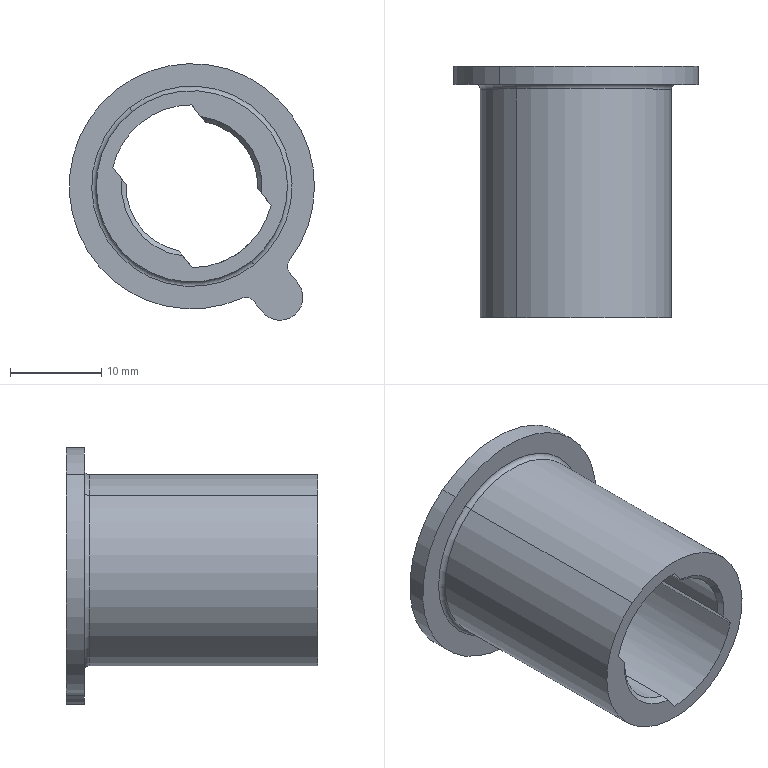Part | SolidWorks | features BaseBody 1 | 1 solid | 36 faces | box 26.8 x 27.5 x 28.043 mm | volume 3609 mm3 | cylinder 15 | plane 9 | cone 8 | torus 2 | sphere 2 | commonest cylinder face diameters 17.8 x3 2 x2 5 x2 14.4 x2 18 x2 20.9 x2
STEP:
#1=CARTESIAN_POINT('',(223.907,99.5,7.051));
#2=VERTEX_POINT('',#1);
#3=CARTESIAN_POINT('',(235.093,99.5,-7.051));
#4=VERTEX_POINT('',#3);
#5=CARTESIAN_POINT('',(229.5,99.5,0.));
#6=DIRECTION('',(0.,1.,0.));
#7=DIRECTION('',(0.6215,0.,-0.7834));
#8=AXIS2_PLACEMENT_3D('',#5,#6,#7);
#9=CIRCLE('',#8,9.);
#10=EDGE_CURVE('',#2,#4,#9,.T.);
#11=ORIENTED_EDGE('',*,*,#10,.F.);
#12=CARTESIAN_POINT('',(223.596,100.,7.443));
#13=VERTEX_POINT('',#12);
#14=CARTESIAN_POINT('',(223.596,100.,7.443));
#15=DIRECTION('',(-0.4395,0.7071,0.554));
#16=VECTOR('',#15,1000.);
#17=LINE('',#14,#16);
#18=EDGE_CURVE('',#2,#13,#17,.T.);
#19=ORIENTED_EDGE('',*,*,#18,.T.);
#20=CARTESIAN_POINT('',(235.404,100.,-7.443));
#21=VERTEX_POINT('',#20);
#22=CARTESIAN_POINT('',(229.5,100.,0.));
#23=DIRECTION('',(0.,-1.,0.));
#24=DIRECTION('',(0.6215,0.,-0.7834));
#25=AXIS2_PLACEMENT_3D('',#22,#23,#24);
#26=CIRCLE('',#25,9.5);
#27=EDGE_CURVE('',#21,#13,#26,.T.);
#28=ORIENTED_EDGE('',*,*,#27,.F.);
#29=CARTESIAN_POINT('',(235.404,100.,-7.443));
#30=DIRECTION('',(0.4395,0.7071,-0.554));
#31=VECTOR('',#30,1000.);
#32=LINE('',#29,#31);
#33=EDGE_CURVE('',#4,#21,#32,.T.);
#34=ORIENTED_EDGE('',*,*,#33,.F.);
#35=EDGE_LOOP('',(#11,#19,#28,#34));
#36=FACE_OUTER_BOUND('',#35,.T.);
#37=CARTESIAN_POINT('',(229.5,100.,0.));
#38=DIRECTION('',(0.,1.,0.));
#39=DIRECTION('',(0.6215,0.,-0.7834));
#40=AXIS2_PLACEMENT_3D('',#37,#38,#39);
#41=CONICAL_SURFACE('',#40,9.5,0.7854);
#42=ADVANCED_FACE('',(#36),#41,.F.);
#43=CARTESIAN_POINT('',(235.995,97.5,-8.187));
#44=VERTEX_POINT('',#43);
#45=CARTESIAN_POINT('',(223.005,97.5,8.187));
#46=VERTEX_POINT('',#45);
#47=CARTESIAN_POINT('',(229.5,97.5,0.));
#48=DIRECTION('',(0.,-1.,0.));
#49=DIRECTION('',(-0.6215,0.,0.7834));
#50=AXIS2_PLACEMENT_3D('',#47,#48,#49);
#51=CIRCLE('',#50,10.45);
#52=EDGE_CURVE('',#44,#46,#51,.T.);
#53=ORIENTED_EDGE('',*,*,#52,.F.);
#54=CARTESIAN_POINT('',(236.305,98.,-8.578));
#55=VERTEX_POINT('',#54);
#56=CARTESIAN_POINT('',(236.305,97.5,-8.578));
#57=DIRECTION('',(-0.7834,0.,-0.6215));
#58=DIRECTION('',(-0.6215,0.,0.7834));
#59=AXIS2_PLACEMENT_3D('',#56,#57,#58);
#60=CIRCLE('',#59,0.5);
#61=EDGE_CURVE('',#44,#55,#60,.T.);
#62=ORIENTED_EDGE('',*,*,#61,.T.);
#63=CARTESIAN_POINT('',(222.695,98.,8.578));
#64=VERTEX_POINT('',#63);
#65=CARTESIAN_POINT('',(229.5,98.,0.));
#66=DIRECTION('',(0.,1.,0.));
#67=DIRECTION('',(-0.6215,0.,0.7834));
#68=AXIS2_PLACEMENT_3D('',#65,#66,#67);
#69=CIRCLE('',#68,10.95);
#70=EDGE_CURVE('',#64,#55,#69,.T.);
#71=ORIENTED_EDGE('',*,*,#70,.F.);
#72=CARTESIAN_POINT('',(222.695,97.5,8.578));
#73=DIRECTION('',(0.7834,0.,0.6215));
#74=DIRECTION('',(0.6215,0.,-0.7834));
#75=AXIS2_PLACEMENT_3D('',#72,#73,#74);
#76=CIRCLE('',#75,0.5);
#77=EDGE_CURVE('',#46,#64,#76,.T.);
#78=ORIENTED_EDGE('',*,*,#77,.F.);
#79=EDGE_LOOP('',(#53,#62,#71,#78));
#80=FACE_OUTER_BOUND('',#79,.T.);
#81=CARTESIAN_POINT('',(229.5,97.5,0.));
#82=DIRECTION('',(0.,-1.,0.));
#83=DIRECTION('',(-0.6215,0.,0.7834));
#84=AXIS2_PLACEMENT_3D('',#81,#82,#83);
#85=TOROIDAL_SURFACE('',#84,10.95,0.5);
#86=ADVANCED_FACE('',(#80),#85,.F.);
#87=CARTESIAN_POINT('',(239.133,99.5,-12.143));
#88=VERTEX_POINT('',#87);
#89=CARTESIAN_POINT('',(240.065,100.,-13.318));
#90=VERTEX_POINT('',#89);
#91=CARTESIAN_POINT('',(239.133,102.,-12.143));
#92=DIRECTION('',(0.7834,0.,0.6215));
#93=DIRECTION('',(0.6215,0.,-0.7834));
#94=AXIS2_PLACEMENT_3D('',#91,#92,#93);
#95=CIRCLE('',#94,2.5);
#96=EDGE_CURVE('',#88,#90,#95,.T.);
#97=ORIENTED_EDGE('',*,*,#96,.F.);
#98=CARTESIAN_POINT('',(238.201,100.,-10.968));
#99=VERTEX_POINT('',#98);
#100=CARTESIAN_POINT('',(239.133,102.,-12.143));
#101=DIRECTION('',(-0.7834,0.,-0.6215));
#102=DIRECTION('',(-0.6215,0.,0.7834));
#103=AXIS2_PLACEMENT_3D('',#100,#101,#102);
#104=CIRCLE('',#103,2.5);
#105=EDGE_CURVE('',#88,#99,#104,.T.);
#106=ORIENTED_EDGE('',*,*,#105,.T.);
#107=CARTESIAN_POINT('',(239.133,100.,-12.143));
#108=DIRECTION('',(0.,1.,0.));
#109=DIRECTION('',(0.6215,0.,-0.7834));
#110=AXIS2_PLACEMENT_3D('',#107,#108,#109);
#111=CIRCLE('',#110,1.5);
#112=EDGE_CURVE('',#99,#90,#111,.T.);
#113=ORIENTED_EDGE('',*,*,#112,.T.);
#114=EDGE_LOOP('',(#97,#106,#113));
#115=FACE_OUTER_BOUND('',#114,.T.);
#116=CARTESIAN_POINT('',(239.133,102.,-12.143));
#117=DIRECTION('',(-0.7834,0.,-0.6215));
#118=DIRECTION('',(0.6215,0.,-0.7834));
#119=AXIS2_PLACEMENT_3D('',#116,#117,#118);
#120=SPHERICAL_SURFACE('',#119,2.5);
#121=ADVANCED_FACE('',(#115),#120,.F.);
#122=CARTESIAN_POINT('',(220.843,86.8,2.064));
#123=VERTEX_POINT('',#122);
#124=CARTESIAN_POINT('',(223.969,86.8,6.972));
#125=VERTEX_POINT('',#124);
#126=CARTESIAN_POINT('',(229.5,86.8,0.));
#127=DIRECTION('',(0.,1.,0.));
#128=DIRECTION('',(0.6215,0.,-0.7834));
#129=AXIS2_PLACEMENT_3D('',#126,#127,#128);
#130=CIRCLE('',#129,8.9);
#131=EDGE_CURVE('',#123,#125,#130,.T.);
#132=ORIENTED_EDGE('',*,*,#131,.T.);
#133=CARTESIAN_POINT('',(223.969,72.5,6.972));
#134=VERTEX_POINT('',#133);
#135=CARTESIAN_POINT('',(223.969,100.,6.972));
#136=DIRECTION('',(0.,-1.,0.));
#137=VECTOR('',#136,1000.);
#138=LINE('',#135,#137);
#139=EDGE_CURVE('',#125,#134,#138,.T.);
#140=ORIENTED_EDGE('',*,*,#139,.T.);
#141=CARTESIAN_POINT('',(220.843,72.5,2.064));
#142=VERTEX_POINT('',#141);
#143=CARTESIAN_POINT('',(229.5,72.5,0.));
#144=DIRECTION('',(0.,-1.,0.));
#145=DIRECTION('',(-0.6215,0.,0.7834));
#146=AXIS2_PLACEMENT_3D('',#143,#144,#145);
#147=CIRCLE('',#146,8.9);
#148=EDGE_CURVE('',#134,#142,#147,.T.);
#149=ORIENTED_EDGE('',*,*,#148,.T.);
#150=CARTESIAN_POINT('',(220.843,100.,2.064));
#151=DIRECTION('',(0.,-1.,0.));
#152=VECTOR('',#151,1000.);
#153=LINE('',#150,#152);
#154=EDGE_CURVE('',#123,#142,#153,.T.);
#155=ORIENTED_EDGE('',*,*,#154,.F.);
#156=EDGE_LOOP('',(#132,#140,#149,#155));
#157=FACE_OUTER_BOUND('',#156,.T.);
#158=CARTESIAN_POINT('',(229.5,100.,0.));
#159=DIRECTION('',(0.,-1.,0.));
#160=DIRECTION('',(-0.6215,0.,0.7834));
#161=AXIS2_PLACEMENT_3D('',#158,#159,#160);
#162=CYLINDRICAL_SURFACE('',#161,8.9);
#163=ADVANCED_FACE('',(#157),#162,.F.);
#164=CARTESIAN_POINT('',(241.092,98.,-10.589));
#165=VERTEX_POINT('',#164);
#166=CARTESIAN_POINT('',(240.687,98.,-14.102));
#167=VERTEX_POINT('',#166);
#168=CARTESIAN_POINT('',(239.133,98.,-12.143));
#169=DIRECTION('',(0.,1.,0.));
#170=DIRECTION('',(-0.6215,0.,0.7834));
#171=AXIS2_PLACEMENT_3D('',#168,#169,#170);
#172=CIRCLE('',#171,2.5);
#173=EDGE_CURVE('',#165,#167,#172,.T.);
#174=ORIENTED_EDGE('',*,*,#173,.T.);
#175=CARTESIAN_POINT('',(240.687,100.,-14.102));
#176=VERTEX_POINT('',#175);
#177=CARTESIAN_POINT('',(240.687,56.718,-14.102));
#178=DIRECTION('',(0.,1.,0.));
#179=VECTOR('',#178,1000.);
#180=LINE('',#177,#179);
#181=EDGE_CURVE('',#167,#176,#180,.T.);
#182=ORIENTED_EDGE('',*,*,#181,.T.);
#183=CARTESIAN_POINT('',(241.092,100.,-10.589));
#184=VERTEX_POINT('',#183);
#185=CARTESIAN_POINT('',(239.133,100.,-12.143));
#186=DIRECTION('',(0.,1.,0.));
#187=DIRECTION('',(-0.6215,0.,0.7834));
#188=AXIS2_PLACEMENT_3D('',#185,#186,#187);
#189=CIRCLE('',#188,2.5);
#190=EDGE_CURVE('',#184,#176,#189,.T.);
#191=ORIENTED_EDGE('',*,*,#190,.F.);
#192=CARTESIAN_POINT('',(241.092,56.718,-10.589));
#193=DIRECTION('',(0.,1.,0.));
#194=VECTOR('',#193,1000.);
#195=LINE('',#192,#194);
#196=EDGE_CURVE('',#165,#184,#195,.T.);
#197=ORIENTED_EDGE('',*,*,#196,.F.);
#198=EDGE_LOOP('',(#174,#182,#191,#197));
#199=FACE_OUTER_BOUND('',#198,.T.);
#200=CARTESIAN_POINT('',(239.133,56.718,-12.143));
#201=DIRECTION('',(0.,1.,0.));
#202=DIRECTION('',(0.6215,0.,-0.7834));
#203=AXIS2_PLACEMENT_3D('',#200,#201,#202);
#204=CYLINDRICAL_SURFACE('',#203,2.5);
#205=ADVANCED_FACE('',(#199),#204,.T.);
#206=CARTESIAN_POINT('',(229.46,86.8,8.9));
#207=VERTEX_POINT('',#206);
#208=CARTESIAN_POINT('',(229.5,86.8,0.));
#209=DIRECTION('',(0.,1.,0.));
#210=DIRECTION('',(0.6215,0.,-0.7834));
#211=AXIS2_PLACEMENT_3D('',#208,#209,#210);
#212=CIRCLE('',#211,8.9);
#213=EDGE_CURVE('',#125,#207,#212,.T.);
#214=ORIENTED_EDGE('',*,*,#213,.F.);
#215=CARTESIAN_POINT('',(223.907,86.9,7.051));
#216=VERTEX_POINT('',#215);
#217=CARTESIAN_POINT('',(223.907,86.9,7.051));
#218=DIRECTION('',(-0.4395,0.7071,0.554));
#219=VECTOR('',#218,1000.);
#220=LINE('',#217,#219);
#221=EDGE_CURVE('',#125,#216,#220,.T.);
#222=ORIENTED_EDGE('',*,*,#221,.T.);
#223=CARTESIAN_POINT('',(235.093,86.9,-7.051));
#224=VERTEX_POINT('',#223);
#225=CARTESIAN_POINT('',(229.5,86.9,0.));
#226=DIRECTION('',(0.,-1.,0.));
#227=DIRECTION('',(-0.6215,0.,0.7834));
#228=AXIS2_PLACEMENT_3D('',#225,#226,#227);
#229=CIRCLE('',#228,9.);
#230=EDGE_CURVE('',#224,#216,#229,.T.);
#231=ORIENTED_EDGE('',*,*,#230,.F.);
#232=CARTESIAN_POINT('',(235.031,86.8,-6.972));
#233=VERTEX_POINT('',#232);
#234=CARTESIAN_POINT('',(235.093,86.9,-7.051));
#235=DIRECTION('',(0.4395,0.7071,-0.554));
#236=VECTOR('',#235,1000.);
#237=LINE('',#234,#236);
#238=EDGE_CURVE('',#233,#224,#237,.T.);
#239=ORIENTED_EDGE('',*,*,#238,.F.);
#240=CARTESIAN_POINT('',(238.157,86.8,-2.064));
#241=VERTEX_POINT('',#240);
#242=CARTESIAN_POINT('',(229.5,86.8,0.));
#243=DIRECTION('',(0.,1.,0.));
#244=DIRECTION('',(0.6215,0.,-0.7834));
#245=AXIS2_PLACEMENT_3D('',#242,#243,#244);
#246=CIRCLE('',#245,8.9);
#247=EDGE_CURVE('',#241,#233,#246,.T.);
#248=ORIENTED_EDGE('',*,*,#247,.F.);
#249=CARTESIAN_POINT('',(237.998,86.6,-1.863));
#250=VERTEX_POINT('',#249);
#251=CARTESIAN_POINT('',(237.998,86.6,-1.863));
#252=CARTESIAN_POINT('',(238.051,86.666,-1.93));
#253=CARTESIAN_POINT('',(238.105,86.733,-1.997));
#254=CARTESIAN_POINT('',(238.157,86.8,-2.064));
#255=B_SPLINE_CURVE_WITH_KNOTS('',3,(#251,#252,#253,#254),.UNSPECIFIED.,.F.,.F.,(4,4),(0.004277,0.004601),.UNSPECIFIED.);
#256=EDGE_CURVE('',#250,#241,#255,.T.);
#257=ORIENTED_EDGE('',*,*,#256,.F.);
#258=CARTESIAN_POINT('',(229.619,86.6,8.699));
#259=VERTEX_POINT('',#258);
#260=CARTESIAN_POINT('',(229.5,86.6,0.));
#261=DIRECTION('',(0.,-1.,0.));
#262=DIRECTION('',(-0.6215,0.,0.7834));
#263=AXIS2_PLACEMENT_3D('',#260,#261,#262);
#264=CIRCLE('',#263,8.7);
#265=EDGE_CURVE('',#250,#259,#264,.T.);
#266=ORIENTED_EDGE('',*,*,#265,.T.);
#267=CARTESIAN_POINT('',(229.46,86.8,8.9));
#268=CARTESIAN_POINT('',(229.513,86.733,8.833));
#269=CARTESIAN_POINT('',(229.566,86.666,8.766));
#270=CARTESIAN_POINT('',(229.619,86.6,8.699));
#271=B_SPLINE_CURVE_WITH_KNOTS('',3,(#267,#268,#269,#270),.UNSPECIFIED.,.F.,.F.,(4,4),(0.004066,0.00439),.UNSPECIFIED.);
#272=EDGE_CURVE('',#207,#259,#271,.T.);
#273=ORIENTED_EDGE('',*,*,#272,.F.);
#274=EDGE_LOOP('',(#214,#222,#231,#239,#248,#257,#266,#273));
#275=FACE_OUTER_BOUND('',#274,.T.);
#276=CARTESIAN_POINT('',(229.5,86.9,0.));
#277=DIRECTION('',(0.,1.,0.));
#278=DIRECTION('',(0.6215,0.,-0.7834));
#279=AXIS2_PLACEMENT_3D('',#276,#277,#278);
#280=CONICAL_SURFACE('',#279,9.,0.7854);
#281=ADVANCED_FACE('',(#275),#280,.F.);
#282=ORIENTED_EDGE('',*,*,#10,.T.);
#283=CARTESIAN_POINT('',(235.093,72.5,-7.051));
#284=DIRECTION('',(0.,-1.,0.));
#285=VECTOR('',#284,1000.);
#286=LINE('',#283,#285);
#287=EDGE_CURVE('',#4,#224,#286,.T.);
#288=ORIENTED_EDGE('',*,*,#287,.T.);
#289=ORIENTED_EDGE('',*,*,#230,.T.);
#290=CARTESIAN_POINT('',(223.907,72.5,7.051));
#291=DIRECTION('',(0.,-1.,0.));
#292=VECTOR('',#291,1000.);
#293=LINE('',#290,#292);
#294=EDGE_CURVE('',#2,#216,#293,.T.);
#295=ORIENTED_EDGE('',*,*,#294,.F.);
#296=EDGE_LOOP('',(#282,#288,#289,#295));
#297=FACE_OUTER_BOUND('',#296,.T.);
#298=CARTESIAN_POINT('',(229.5,72.5,0.));
#299=DIRECTION('',(0.,-1.,0.));
#300=DIRECTION('',(-0.6215,0.,0.7834));
#301=AXIS2_PLACEMENT_3D('',#298,#299,#300);
#302=CYLINDRICAL_SURFACE('',#301,9.);
#303=ADVANCED_FACE('',(#297),#302,.F.);
#304=CARTESIAN_POINT('',(240.13,100.,-8.159));
#305=VERTEX_POINT('',#304);
#306=CARTESIAN_POINT('',(221.172,100.,10.498));
#307=VERTEX_POINT('',#306);
#308=CARTESIAN_POINT('',(229.5,100.,0.));
#309=DIRECTION('',(0.,-1.,0.));
#310=DIRECTION('',(-0.6215,0.,0.7834));
#311=AXIS2_PLACEMENT_3D('',#308,#309,#310);
#312=CIRCLE('',#311,13.4);
#313=EDGE_CURVE('',#305,#307,#312,.T.);
#314=ORIENTED_EDGE('',*,*,#313,.T.);
#315=CARTESIAN_POINT('',(221.172,98.,10.498));
#316=VERTEX_POINT('',#315);
#317=CARTESIAN_POINT('',(221.172,72.5,10.498));
#318=DIRECTION('',(0.,-1.,0.));
#319=VECTOR('',#318,1000.);
#320=LINE('',#317,#319);
#321=EDGE_CURVE('',#307,#316,#320,.T.);
#322=ORIENTED_EDGE('',*,*,#321,.T.);
#323=CARTESIAN_POINT('',(240.13,98.,-8.159));
#324=VERTEX_POINT('',#323);
#325=CARTESIAN_POINT('',(229.5,98.,0.));
#326=DIRECTION('',(0.,-1.,0.));
#327=DIRECTION('',(-0.6215,0.,0.7834));
#328=AXIS2_PLACEMENT_3D('',#325,#326,#327);
#329=CIRCLE('',#328,13.4);
#330=EDGE_CURVE('',#324,#316,#329,.T.);
#331=ORIENTED_EDGE('',*,*,#330,.F.);
#332=CARTESIAN_POINT('',(240.13,72.5,-8.159));
#333=DIRECTION('',(0.,1.,0.));
#334=VECTOR('',#333,1000.);
#335=LINE('',#332,#334);
#336=EDGE_CURVE('',#324,#305,#335,.T.);
#337=ORIENTED_EDGE('',*,*,#336,.T.);
#338=EDGE_LOOP('',(#314,#322,#331,#337));
#339=FACE_OUTER_BOUND('',#338,.T.);
#340=CARTESIAN_POINT('',(229.5,72.5,0.));
#341=DIRECTION('',(0.,-1.,0.));
#342=DIRECTION('',(-0.6215,0.,0.7834));
#343=AXIS2_PLACEMENT_3D('',#340,#341,#342);
#344=CYLINDRICAL_SURFACE('',#343,13.4);
#345=ADVANCED_FACE('',(#339),#344,.T.);
#346=CARTESIAN_POINT('',(229.5,97.5,0.));
#347=DIRECTION('',(0.,-1.,0.));
#348=DIRECTION('',(-0.6215,0.,0.7834));
#349=AXIS2_PLACEMENT_3D('',#346,#347,#348);
#350=CIRCLE('',#349,10.45);
#351=EDGE_CURVE('',#46,#44,#350,.T.);
#352=ORIENTED_EDGE('',*,*,#351,.T.);
#353=CARTESIAN_POINT('',(235.995,72.5,-8.187));
#354=VERTEX_POINT('',#353);
#355=CARTESIAN_POINT('',(235.995,72.5,-8.187));
#356=DIRECTION('',(0.,-1.,0.));
#357=VECTOR('',#356,1000.);
#358=LINE('',#355,#357);
#359=EDGE_CURVE('',#44,#354,#358,.T.);
#360=ORIENTED_EDGE('',*,*,#359,.T.);
#361=CARTESIAN_POINT('',(223.005,72.5,8.187));
#362=VERTEX_POINT('',#361);
#363=CARTESIAN_POINT('',(229.5,72.5,0.));
#364=DIRECTION('',(0.,-1.,0.));
#365=DIRECTION('',(-0.6215,0.,0.7834));
#366=AXIS2_PLACEMENT_3D('',#363,#364,#365);
#367=CIRCLE('',#366,10.45);
#368=EDGE_CURVE('',#362,#354,#367,.T.);
#369=ORIENTED_EDGE('',*,*,#368,.F.);
#370=CARTESIAN_POINT('',(223.005,72.5,8.187));
#371=DIRECTION('',(0.,-1.,0.));
#372=VECTOR('',#371,1000.);
#373=LINE('',#370,#372);
#374=EDGE_CURVE('',#46,#362,#373,.T.);
#375=ORIENTED_EDGE('',*,*,#374,.F.);
#376=EDGE_LOOP('',(#352,#360,#369,#375));
#377=FACE_OUTER_BOUND('',#376,.T.);
#378=CARTESIAN_POINT('',(229.5,72.5,0.));
#379=DIRECTION('',(0.,-1.,0.));
#380=DIRECTION('',(-0.6215,0.,0.7834));
#381=AXIS2_PLACEMENT_3D('',#378,#379,#380);
#382=CYLINDRICAL_SURFACE('',#381,10.45);
#383=ADVANCED_FACE('',(#377),#382,.T.);
#384=CARTESIAN_POINT('',(222.303,85.734,0.222));
#385=VERTEX_POINT('',#384);
#386=CARTESIAN_POINT('',(222.303,73.,0.222));
#387=VERTEX_POINT('',#386);
#388=CARTESIAN_POINT('',(222.303,100.,0.222));
#389=DIRECTION('',(0.,-1.,0.));
#390=VECTOR('',#389,1000.);
#391=LINE('',#388,#390);
#392=EDGE_CURVE('',#385,#387,#391,.T.);
#393=ORIENTED_EDGE('',*,*,#392,.T.);
#394=CARTESIAN_POINT('',(228.079,73.,-7.058));
#395=VERTEX_POINT('',#394);
#396=CARTESIAN_POINT('',(229.5,73.,0.));
#397=DIRECTION('',(0.,-1.,0.));
#398=DIRECTION('',(-0.6215,0.,0.7834));
#399=AXIS2_PLACEMENT_3D('',#396,#397,#398);
#400=CIRCLE('',#399,7.2);
#401=EDGE_CURVE('',#387,#395,#400,.T.);
#402=ORIENTED_EDGE('',*,*,#401,.T.);
#403=CARTESIAN_POINT('',(228.079,85.734,-7.058));
#404=VERTEX_POINT('',#403);
#405=CARTESIAN_POINT('',(228.079,100.,-7.058));
#406=DIRECTION('',(0.,-1.,0.));
#407=VECTOR('',#406,1000.);
#408=LINE('',#405,#407);
#409=EDGE_CURVE('',#404,#395,#408,.T.);
#410=ORIENTED_EDGE('',*,*,#409,.F.);
#411=CARTESIAN_POINT('',(229.5,85.734,0.));
#412=DIRECTION('',(0.,-1.,0.));
#413=DIRECTION('',(-0.6215,0.,0.7834));
#414=AXIS2_PLACEMENT_3D('',#411,#412,#413);
#415=CIRCLE('',#414,7.2);
#416=EDGE_CURVE('',#385,#404,#415,.T.);
#417=ORIENTED_EDGE('',*,*,#416,.F.);
#418=EDGE_LOOP('',(#393,#402,#410,#417));
#419=FACE_OUTER_BOUND('',#418,.T.);
#420=CARTESIAN_POINT('',(229.5,72.5,0.));
#421=DIRECTION('',(0.,-1.,0.));
#422=DIRECTION('',(-0.6215,0.,0.7834));
#423=AXIS2_PLACEMENT_3D('',#420,#421,#422);
#424=CYLINDRICAL_SURFACE('',#423,7.2);
#425=ADVANCED_FACE('',(#419),#424,.F.);
#426=CARTESIAN_POINT('',(229.381,86.6,-8.699));
#427=VERTEX_POINT('',#426);
#428=CARTESIAN_POINT('',(229.381,86.6,-8.699));
#429=CARTESIAN_POINT('',(228.952,86.292,-8.159));
#430=CARTESIAN_POINT('',(228.519,85.997,-7.612));
#431=CARTESIAN_POINT('',(228.079,85.734,-7.058));
#432=B_SPLINE_CURVE_WITH_KNOTS('',3,(#428,#429,#430,#431),.UNSPECIFIED.,.F.,.F.,(4,4),(0.003137,0.005403),.UNSPECIFIED.);
#433=EDGE_CURVE('',#427,#404,#432,.T.);
#434=ORIENTED_EDGE('',*,*,#433,.F.);
#435=CARTESIAN_POINT('',(221.002,86.6,1.863));
#436=VERTEX_POINT('',#435);
#437=CARTESIAN_POINT('',(229.5,86.6,0.));
#438=DIRECTION('',(0.,-1.,0.));
#439=DIRECTION('',(-0.6215,0.,0.7834));
#440=AXIS2_PLACEMENT_3D('',#437,#438,#439);
#441=CIRCLE('',#440,8.7);
#442=EDGE_CURVE('',#436,#427,#441,.T.);
#443=ORIENTED_EDGE('',*,*,#442,.F.);
#444=CARTESIAN_POINT('',(222.303,85.734,0.222));
#445=CARTESIAN_POINT('',(221.864,85.997,0.7756));
#446=CARTESIAN_POINT('',(221.431,86.291,1.322));
#447=CARTESIAN_POINT('',(221.002,86.6,1.863));
#448=B_SPLINE_CURVE_WITH_KNOTS('',3,(#444,#445,#446,#447),.UNSPECIFIED.,.F.,.F.,(4,4),(0.002935,0.005196),.UNSPECIFIED.);
#449=EDGE_CURVE('',#385,#436,#448,.T.);
#450=ORIENTED_EDGE('',*,*,#449,.F.);
#451=ORIENTED_EDGE('',*,*,#416,.T.);
#452=EDGE_LOOP('',(#434,#443,#450,#451));
#453=FACE_OUTER_BOUND('',#452,.T.);
#454=CARTESIAN_POINT('',(229.5,86.6,0.));
#455=DIRECTION('',(0.,1.,0.));
#456=DIRECTION('',(0.6215,0.,-0.7834));
#457=AXIS2_PLACEMENT_3D('',#454,#455,#456);
#458=CONICAL_SURFACE('',#457,8.7,1.047);
#459=ADVANCED_FACE('',(#453),#458,.F.);
#460=CARTESIAN_POINT('',(236.697,85.734,-0.222));
#461=VERTEX_POINT('',#460);
#462=CARTESIAN_POINT('',(236.697,73.,-0.222));
#463=VERTEX_POINT('',#462);
#464=CARTESIAN_POINT('',(236.697,100.,-0.222));
#465=DIRECTION('',(0.,-1.,0.));
#466=VECTOR('',#465,1000.);
#467=LINE('',#464,#466);
#468=EDGE_CURVE('',#461,#463,#467,.T.);
#469=ORIENTED_EDGE('',*,*,#468,.T.);
#470=CARTESIAN_POINT('',(230.921,73.,7.058));
#471=VERTEX_POINT('',#470);
#472=CARTESIAN_POINT('',(229.5,73.,0.));
#473=DIRECTION('',(0.,-1.,0.));
#474=DIRECTION('',(-0.6215,0.,0.7834));
#475=AXIS2_PLACEMENT_3D('',#472,#473,#474);
#476=CIRCLE('',#475,7.2);
#477=EDGE_CURVE('',#463,#471,#476,.T.);
#478=ORIENTED_EDGE('',*,*,#477,.T.);
#479=CARTESIAN_POINT('',(230.921,85.734,7.058));
#480=VERTEX_POINT('',#479);
#481=CARTESIAN_POINT('',(230.921,100.,7.058));
#482=DIRECTION('',(0.,-1.,0.));
#483=VECTOR('',#482,1000.);
#484=LINE('',#481,#483);
#485=EDGE_CURVE('',#480,#471,#484,.T.);
#486=ORIENTED_EDGE('',*,*,#485,.F.);
#487=CARTESIAN_POINT('',(229.5,85.734,0.));
#488=DIRECTION('',(0.,-1.,0.));
#489=DIRECTION('',(-0.6215,0.,0.7834));
#490=AXIS2_PLACEMENT_3D('',#487,#488,#489);
#491=CIRCLE('',#490,7.2);
#492=EDGE_CURVE('',#461,#480,#491,.T.);
#493=ORIENTED_EDGE('',*,*,#492,.F.);
#494=EDGE_LOOP('',(#469,#478,#486,#493));
#495=FACE_OUTER_BOUND('',#494,.T.);
#496=CARTESIAN_POINT('',(229.5,72.5,0.));
#497=DIRECTION('',(0.,-1.,0.));
#498=DIRECTION('',(-0.6215,0.,0.7834));
#499=AXIS2_PLACEMENT_3D('',#496,#497,#498);
#500=CYLINDRICAL_SURFACE('',#499,7.2);
#501=ADVANCED_FACE('',(#495),#500,.F.);
#502=CARTESIAN_POINT('',(230.46,72.5,7.64));
#503=VERTEX_POINT('',#502);
#504=CARTESIAN_POINT('',(229.46,72.5,8.9));
#505=VERTEX_POINT('',#504);
#506=CARTESIAN_POINT('',(230.921,72.5,7.058));
#507=DIRECTION('',(-0.6215,0.,0.7834));
#508=VECTOR('',#507,1000.);
#509=LINE('',#506,#508);
#510=EDGE_CURVE('',#503,#505,#509,.T.);
#511=ORIENTED_EDGE('',*,*,#510,.F.);
#512=CARTESIAN_POINT('',(237.158,72.5,-0.8036));
#513=VERTEX_POINT('',#512);
#514=CARTESIAN_POINT('',(229.5,72.5,0.));
#515=DIRECTION('',(0.,1.,0.));
#516=DIRECTION('',(-0.6215,0.,0.7834));
#517=AXIS2_PLACEMENT_3D('',#514,#515,#516);
#518=CIRCLE('',#517,7.7);
#519=EDGE_CURVE('',#503,#513,#518,.T.);
#520=ORIENTED_EDGE('',*,*,#519,.T.);
#521=CARTESIAN_POINT('',(238.157,72.5,-2.064));
#522=VERTEX_POINT('',#521);
#523=CARTESIAN_POINT('',(236.697,72.5,-0.222));
#524=DIRECTION('',(-0.6215,0.,0.7834));
#525=VECTOR('',#524,1000.);
#526=LINE('',#523,#525);
#527=EDGE_CURVE('',#522,#513,#526,.T.);
#528=ORIENTED_EDGE('',*,*,#527,.F.);
#529=CARTESIAN_POINT('',(229.54,72.5,-8.9));
#530=VERTEX_POINT('',#529);
#531=CARTESIAN_POINT('',(229.5,72.5,0.));
#532=DIRECTION('',(0.,-1.,0.));
#533=DIRECTION('',(-0.6215,0.,0.7834));
#534=AXIS2_PLACEMENT_3D('',#531,#532,#533);
#535=CIRCLE('',#534,8.9);
#536=EDGE_CURVE('',#530,#522,#535,.T.);
#537=ORIENTED_EDGE('',*,*,#536,.F.);
#538=CARTESIAN_POINT('',(228.54,72.5,-7.64));
#539=VERTEX_POINT('',#538);
#540=CARTESIAN_POINT('',(228.079,72.5,-7.058));
#541=DIRECTION('',(0.6215,0.,-0.7834));
#542=VECTOR('',#541,1000.);
#543=LINE('',#540,#542);
#544=EDGE_CURVE('',#539,#530,#543,.T.);
#545=ORIENTED_EDGE('',*,*,#544,.F.);
#546=CARTESIAN_POINT('',(221.842,72.5,0.8036));
#547=VERTEX_POINT('',#546);
#548=CARTESIAN_POINT('',(229.5,72.5,0.));
#549=DIRECTION('',(0.,1.,0.));
#550=DIRECTION('',(-0.6215,0.,0.7834));
#551=AXIS2_PLACEMENT_3D('',#548,#549,#550);
#552=CIRCLE('',#551,7.7);
#553=EDGE_CURVE('',#539,#547,#552,.T.);
#554=ORIENTED_EDGE('',*,*,#553,.T.);
#555=CARTESIAN_POINT('',(222.303,72.5,0.222));
#556=DIRECTION('',(0.6215,0.,-0.7834));
#557=VECTOR('',#556,1000.);
#558=LINE('',#555,#557);
#559=EDGE_CURVE('',#142,#547,#558,.T.);
#560=ORIENTED_EDGE('',*,*,#559,.F.);
#561=ORIENTED_EDGE('',*,*,#148,.F.);
#562=CARTESIAN_POINT('',(229.5,72.5,0.));
#563=DIRECTION('',(0.,-1.,0.));
#564=DIRECTION('',(-0.6215,0.,0.7834));
#565=AXIS2_PLACEMENT_3D('',#562,#563,#564);
#566=CIRCLE('',#565,8.9);
#567=EDGE_CURVE('',#505,#134,#566,.T.);
#568=ORIENTED_EDGE('',*,*,#567,.F.);
#569=EDGE_LOOP('',(#511,#520,#528,#537,#545,#554,#560,#561,#568));
#570=FACE_BOUND('',#569,.T.);
#571=ORIENTED_EDGE('',*,*,#368,.T.);
#572=CARTESIAN_POINT('',(229.5,72.5,0.));
#573=DIRECTION('',(0.,-1.,0.));
#574=DIRECTION('',(-0.6215,0.,0.7834));
#575=AXIS2_PLACEMENT_3D('',#572,#573,#574);
#576=CIRCLE('',#575,10.45);
#577=EDGE_CURVE('',#354,#362,#576,.T.);
#578=ORIENTED_EDGE('',*,*,#577,.T.);
#579=EDGE_LOOP('',(#571,#578));
#580=FACE_OUTER_BOUND('',#579,.T.);
#581=CARTESIAN_POINT('',(223.859,72.5,-4.475));
#582=DIRECTION('',(0.,-1.,0.));
#583=DIRECTION('',(-0.6215,0.,0.7834));
#584=AXIS2_PLACEMENT_3D('',#581,#582,#583);
#585=PLANE('',#584);
#586=ADVANCED_FACE('',(#570,#580),#585,.T.);
#587=ORIENTED_EDGE('',*,*,#359,.F.);
#588=ORIENTED_EDGE('',*,*,#52,.T.);
#589=ORIENTED_EDGE('',*,*,#374,.T.);
#590=ORIENTED_EDGE('',*,*,#577,.F.);
#591=EDGE_LOOP('',(#587,#588,#589,#590));
#592=FACE_OUTER_BOUND('',#591,.T.);
#593=CARTESIAN_POINT('',(229.5,72.5,0.));
#594=DIRECTION('',(0.,-1.,0.));
#595=DIRECTION('',(-0.6215,0.,0.7834));
#596=AXIS2_PLACEMENT_3D('',#593,#594,#595);
#597=CYLINDRICAL_SURFACE('',#596,10.45);
#598=ADVANCED_FACE('',(#592),#597,.T.);
#599=ORIENTED_EDGE('',*,*,#70,.T.);
#600=CARTESIAN_POINT('',(229.5,98.,0.));
#601=DIRECTION('',(0.,1.,0.));
#602=DIRECTION('',(-0.6215,0.,0.7834));
#603=AXIS2_PLACEMENT_3D('',#600,#601,#602);
#604=CIRCLE('',#603,10.95);
#605=EDGE_CURVE('',#55,#64,#604,.T.);
#606=ORIENTED_EDGE('',*,*,#605,.T.);
#607=EDGE_LOOP('',(#599,#606));
#608=FACE_BOUND('',#607,.T.);
#609=CARTESIAN_POINT('',(240.14,98.,-9.389));
#610=VERTEX_POINT('',#609);
#611=CARTESIAN_POINT('',(239.64,98.,-8.76));
#612=DIRECTION('',(0.6215,0.,-0.7834));
#613=VECTOR('',#612,1000.);
#614=LINE('',#611,#613);
#615=EDGE_CURVE('',#610,#165,#614,.T.);
#616=ORIENTED_EDGE('',*,*,#615,.F.);
#617=CARTESIAN_POINT('',(240.923,98.,-8.768));
#618=DIRECTION('',(0.,1.,0.));
#619=DIRECTION('',(-0.6215,0.,0.7834));
#620=AXIS2_PLACEMENT_3D('',#617,#618,#619);
#621=CIRCLE('',#620,1.);
#622=EDGE_CURVE('',#610,#324,#621,.T.);
#623=ORIENTED_EDGE('',*,*,#622,.T.);
#624=ORIENTED_EDGE('',*,*,#330,.T.);
#625=CARTESIAN_POINT('',(235.027,98.,-12.207));
#626=VERTEX_POINT('',#625);
#627=CARTESIAN_POINT('',(229.5,98.,0.));
#628=DIRECTION('',(0.,-1.,0.));
#629=DIRECTION('',(-0.6215,0.,0.7834));
#630=AXIS2_PLACEMENT_3D('',#627,#628,#629);
#631=CIRCLE('',#630,13.4);
#632=EDGE_CURVE('',#316,#626,#631,.T.);
#633=ORIENTED_EDGE('',*,*,#632,.T.);
#634=CARTESIAN_POINT('',(236.223,98.,-12.497));
#635=VERTEX_POINT('',#634);
#636=CARTESIAN_POINT('',(235.439,98.,-13.118));
#637=DIRECTION('',(0.,1.,0.));
#638=DIRECTION('',(-0.6215,0.,0.7834));
#639=AXIS2_PLACEMENT_3D('',#636,#637,#638);
#640=CIRCLE('',#639,1.);
#641=EDGE_CURVE('',#626,#635,#640,.T.);
#642=ORIENTED_EDGE('',*,*,#641,.T.);
#643=CARTESIAN_POINT('',(237.175,98.,-13.697));
#644=VERTEX_POINT('',#643);
#645=CARTESIAN_POINT('',(235.723,98.,-11.867));
#646=DIRECTION('',(-0.6215,0.,0.7834));
#647=VECTOR('',#646,1000.);
#648=LINE('',#645,#647);
#649=EDGE_CURVE('',#644,#635,#648,.T.);
#650=ORIENTED_EDGE('',*,*,#649,.F.);
#651=CARTESIAN_POINT('',(239.133,98.,-12.143));
#652=DIRECTION('',(0.,1.,0.));
#653=DIRECTION('',(-0.6215,0.,0.7834));
#654=AXIS2_PLACEMENT_3D('',#651,#652,#653);
#655=CIRCLE('',#654,2.5);
#656=EDGE_CURVE('',#167,#644,#655,.T.);
#657=ORIENTED_EDGE('',*,*,#656,.F.);
#658=ORIENTED_EDGE('',*,*,#173,.F.);
#659=EDGE_LOOP('',(#616,#623,#624,#633,#642,#650,#657,#658));
#660=FACE_OUTER_BOUND('',#659,.T.);
#661=CARTESIAN_POINT('',(221.313,98.,-6.495));
#662=DIRECTION('',(0.,-1.,0.));
#663=DIRECTION('',(-0.6215,0.,0.7834));
#664=AXIS2_PLACEMENT_3D('',#661,#662,#663);
#665=PLANE('',#664);
#666=ADVANCED_FACE('',(#608,#660),#665,.T.);
#667=ORIENTED_EDGE('',*,*,#321,.F.);
#668=CARTESIAN_POINT('',(235.027,100.,-12.207));
#669=VERTEX_POINT('',#668);
#670=CARTESIAN_POINT('',(229.5,100.,0.));
#671=DIRECTION('',(0.,-1.,0.));
#672=DIRECTION('',(-0.6215,0.,0.7834));
#673=AXIS2_PLACEMENT_3D('',#670,#671,#672);
#674=CIRCLE('',#673,13.4);
#675=EDGE_CURVE('',#307,#669,#674,.T.);
#676=ORIENTED_EDGE('',*,*,#675,.T.);
#677=CARTESIAN_POINT('',(235.027,72.5,-12.207));
#678=DIRECTION('',(0.,-1.,0.));
#679=VECTOR('',#678,1000.);
#680=LINE('',#677,#679);
#681=EDGE_CURVE('',#669,#626,#680,.T.);
#682=ORIENTED_EDGE('',*,*,#681,.T.);
#683=ORIENTED_EDGE('',*,*,#632,.F.);
#684=EDGE_LOOP('',(#667,#676,#682,#683));
#685=FACE_OUTER_BOUND('',#684,.T.);
#686=CARTESIAN_POINT('',(229.5,72.5,0.));
#687=DIRECTION('',(0.,-1.,0.));
#688=DIRECTION('',(-0.6215,0.,0.7834));
#689=AXIS2_PLACEMENT_3D('',#686,#687,#688);
#690=CYLINDRICAL_SURFACE('',#689,13.4);
#691=ADVANCED_FACE('',(#685),#690,.T.);
#692=ORIENTED_EDGE('',*,*,#27,.T.);
#693=CARTESIAN_POINT('',(229.5,100.,0.));
#694=DIRECTION('',(0.,-1.,0.));
#695=DIRECTION('',(0.6215,0.,-0.7834));
#696=AXIS2_PLACEMENT_3D('',#693,#694,#695);
#697=CIRCLE('',#696,9.5);
#698=EDGE_CURVE('',#13,#21,#697,.T.);
#699=ORIENTED_EDGE('',*,*,#698,.T.);
#700=EDGE_LOOP('',(#692,#699));
#701=FACE_BOUND('',#700,.T.);
#702=CARTESIAN_POINT('',(239.133,100.,-12.143));
#703=DIRECTION('',(0.,1.,0.));
#704=DIRECTION('',(0.6215,0.,-0.7834));
#705=AXIS2_PLACEMENT_3D('',#702,#703,#704);
#706=CIRCLE('',#705,1.5);
#707=EDGE_CURVE('',#90,#99,#706,.T.);
#708=ORIENTED_EDGE('',*,*,#707,.F.);
#709=ORIENTED_EDGE('',*,*,#112,.F.);
#710=EDGE_LOOP('',(#708,#709));
#711=FACE_BOUND('',#710,.T.);
#712=ORIENTED_EDGE('',*,*,#313,.F.);
#713=CARTESIAN_POINT('',(240.14,100.,-9.389));
#714=VERTEX_POINT('',#713);
#715=CARTESIAN_POINT('',(240.923,100.,-8.768));
#716=DIRECTION('',(0.,-1.,0.));
#717=DIRECTION('',(0.6215,0.,-0.7834));
#718=AXIS2_PLACEMENT_3D('',#715,#716,#717);
#719=CIRCLE('',#718,1.);
#720=EDGE_CURVE('',#305,#714,#719,.T.);
#721=ORIENTED_EDGE('',*,*,#720,.T.);
#722=CARTESIAN_POINT('',(239.64,100.,-8.76));
#723=DIRECTION('',(0.6215,0.,-0.7834));
#724=VECTOR('',#723,1000.);
#725=LINE('',#722,#724);
#726=EDGE_CURVE('',#714,#184,#725,.T.);
#727=ORIENTED_EDGE('',*,*,#726,.T.);
#728=ORIENTED_EDGE('',*,*,#190,.T.);
#729=CARTESIAN_POINT('',(237.175,100.,-13.697));
#730=VERTEX_POINT('',#729);
#731=CARTESIAN_POINT('',(239.133,100.,-12.143));
#732=DIRECTION('',(0.,1.,0.));
#733=DIRECTION('',(-0.6215,0.,0.7834));
#734=AXIS2_PLACEMENT_3D('',#731,#732,#733);
#735=CIRCLE('',#734,2.5);
#736=EDGE_CURVE('',#176,#730,#735,.T.);
#737=ORIENTED_EDGE('',*,*,#736,.T.);
#738=CARTESIAN_POINT('',(236.223,100.,-12.497));
#739=VERTEX_POINT('',#738);
#740=CARTESIAN_POINT('',(235.723,100.,-11.867));
#741=DIRECTION('',(-0.6215,0.,0.7834));
#742=VECTOR('',#741,1000.);
#743=LINE('',#740,#742);
#744=EDGE_CURVE('',#730,#739,#743,.T.);
#745=ORIENTED_EDGE('',*,*,#744,.T.);
#746=CARTESIAN_POINT('',(235.439,100.,-13.118));
#747=DIRECTION('',(0.,-1.,0.));
#748=DIRECTION('',(0.6215,0.,-0.7834));
#749=AXIS2_PLACEMENT_3D('',#746,#747,#748);
#750=CIRCLE('',#749,1.);
#751=EDGE_CURVE('',#739,#669,#750,.T.);
#752=ORIENTED_EDGE('',*,*,#751,.T.);
#753=ORIENTED_EDGE('',*,*,#675,.F.);
#754=EDGE_LOOP('',(#712,#721,#727,#728,#737,#745,#752,#753));
#755=FACE_OUTER_BOUND('',#754,.T.);
#756=CARTESIAN_POINT('',(219.002,100.,-8.328));
#757=DIRECTION('',(0.,1.,0.));
#758=DIRECTION('',(0.6215,0.,-0.7834));
#759=AXIS2_PLACEMENT_3D('',#756,#757,#758);
#760=PLANE('',#759);
#761=ADVANCED_FACE('',(#701,#711,#755),#760,.T.);
#762=ORIENTED_EDGE('',*,*,#287,.F.);
#763=CARTESIAN_POINT('',(229.5,99.5,0.));
#764=DIRECTION('',(0.,1.,0.));
#765=DIRECTION('',(0.6215,0.,-0.7834));
#766=AXIS2_PLACEMENT_3D('',#763,#764,#765);
#767=CIRCLE('',#766,9.);
#768=EDGE_CURVE('',#4,#2,#767,.T.);
#769=ORIENTED_EDGE('',*,*,#768,.T.);
#770=ORIENTED_EDGE('',*,*,#294,.T.);
#771=CARTESIAN_POINT('',(229.5,86.9,0.));
#772=DIRECTION('',(0.,-1.,0.));
#773=DIRECTION('',(-0.6215,0.,0.7834));
#774=AXIS2_PLACEMENT_3D('',#771,#772,#773);
#775=CIRCLE('',#774,9.);
#776=EDGE_CURVE('',#216,#224,#775,.T.);
#777=ORIENTED_EDGE('',*,*,#776,.T.);
#778=EDGE_LOOP('',(#762,#769,#770,#777));
#779=FACE_OUTER_BOUND('',#778,.T.);
#780=CARTESIAN_POINT('',(229.5,72.5,0.));
#781=DIRECTION('',(0.,-1.,0.));
#782=DIRECTION('',(-0.6215,0.,0.7834));
#783=AXIS2_PLACEMENT_3D('',#780,#781,#782);
#784=CYLINDRICAL_SURFACE('',#783,9.);
#785=ADVANCED_FACE('',(#779),#784,.F.);
#786=ORIENTED_EDGE('',*,*,#221,.F.);
#787=ORIENTED_EDGE('',*,*,#131,.F.);
#788=CARTESIAN_POINT('',(221.002,86.6,1.863));
#789=CARTESIAN_POINT('',(220.949,86.666,1.93));
#790=CARTESIAN_POINT('',(220.895,86.733,1.997));
#791=CARTESIAN_POINT('',(220.843,86.8,2.064));
#792=B_SPLINE_CURVE_WITH_KNOTS('',3,(#788,#789,#790,#791),.UNSPECIFIED.,.F.,.F.,(4,4),(0.004277,0.004601),.UNSPECIFIED.);
#793=EDGE_CURVE('',#436,#123,#792,.T.);
#794=ORIENTED_EDGE('',*,*,#793,.F.);
#795=ORIENTED_EDGE('',*,*,#442,.T.);
#796=CARTESIAN_POINT('',(229.54,86.8,-8.9));
#797=VERTEX_POINT('',#796);
#798=CARTESIAN_POINT('',(229.54,86.8,-8.9));
#799=CARTESIAN_POINT('',(229.487,86.733,-8.833));
#800=CARTESIAN_POINT('',(229.434,86.666,-8.766));
#801=CARTESIAN_POINT('',(229.381,86.6,-8.699));
#802=B_SPLINE_CURVE_WITH_KNOTS('',3,(#798,#799,#800,#801),.UNSPECIFIED.,.F.,.F.,(4,4),(0.004066,0.00439),.UNSPECIFIED.);
#803=EDGE_CURVE('',#797,#427,#802,.T.);
#804=ORIENTED_EDGE('',*,*,#803,.F.);
#805=CARTESIAN_POINT('',(229.5,86.8,0.));
#806=DIRECTION('',(0.,1.,0.));
#807=DIRECTION('',(0.6215,0.,-0.7834));
#808=AXIS2_PLACEMENT_3D('',#805,#806,#807);
#809=CIRCLE('',#808,8.9);
#810=EDGE_CURVE('',#233,#797,#809,.T.);
#811=ORIENTED_EDGE('',*,*,#810,.F.);
#812=ORIENTED_EDGE('',*,*,#238,.T.);
#813=ORIENTED_EDGE('',*,*,#776,.F.);
#814=EDGE_LOOP('',(#786,#787,#794,#795,#804,#811,#812,#813));
#815=FACE_OUTER_BOUND('',#814,.T.);
#816=CARTESIAN_POINT('',(229.5,86.9,0.));
#817=DIRECTION('',(0.,1.,0.));
#818=DIRECTION('',(0.6215,0.,-0.7834));
#819=AXIS2_PLACEMENT_3D('',#816,#817,#818);
#820=CONICAL_SURFACE('',#819,9.,0.7854);
#821=ADVANCED_FACE('',(#815),#820,.F.);
#822=CARTESIAN_POINT('',(236.697,85.734,-0.222));
#823=CARTESIAN_POINT('',(237.137,85.998,-0.777));
#824=CARTESIAN_POINT('',(237.57,86.292,-1.323));
#825=CARTESIAN_POINT('',(237.998,86.6,-1.863));
#826=B_SPLINE_CURVE_WITH_KNOTS('',3,(#822,#823,#824,#825),.UNSPECIFIED.,.F.,.F.,(4,4),(0.004592,0.006841),.UNSPECIFIED.);
#827=EDGE_CURVE('',#461,#250,#826,.T.);
#828=ORIENTED_EDGE('',*,*,#827,.F.);
#829=ORIENTED_EDGE('',*,*,#492,.T.);
#830=CARTESIAN_POINT('',(229.619,86.6,8.699));
#831=CARTESIAN_POINT('',(230.049,86.291,8.158));
#832=CARTESIAN_POINT('',(230.482,85.997,7.612));
#833=CARTESIAN_POINT('',(230.921,85.734,7.058));
#834=B_SPLINE_CURVE_WITH_KNOTS('',3,(#830,#831,#832,#833),.UNSPECIFIED.,.F.,.F.,(4,4),(0.004758,0.007027),.UNSPECIFIED.);
#835=EDGE_CURVE('',#259,#480,#834,.T.);
#836=ORIENTED_EDGE('',*,*,#835,.F.);
#837=ORIENTED_EDGE('',*,*,#265,.F.);
#838=EDGE_LOOP('',(#828,#829,#836,#837));
#839=FACE_OUTER_BOUND('',#838,.T.);
#840=CARTESIAN_POINT('',(229.5,86.6,0.));
#841=DIRECTION('',(0.,1.,0.));
#842=DIRECTION('',(0.6215,0.,-0.7834));
#843=AXIS2_PLACEMENT_3D('',#840,#841,#842);
#844=CONICAL_SURFACE('',#843,8.7,1.047);
#845=ADVANCED_FACE('',(#839),#844,.F.);
#846=ORIENTED_EDGE('',*,*,#649,.T.);
#847=CARTESIAN_POINT('',(236.223,100.,-12.497));
#848=DIRECTION('',(0.,1.,0.));
#849=VECTOR('',#848,1000.);
#850=LINE('',#847,#849);
#851=EDGE_CURVE('',#635,#739,#850,.T.);
#852=ORIENTED_EDGE('',*,*,#851,.T.);
#853=ORIENTED_EDGE('',*,*,#744,.F.);
#854=CARTESIAN_POINT('',(237.175,56.718,-13.697));
#855=DIRECTION('',(0.,1.,0.));
#856=VECTOR('',#855,1000.);
#857=LINE('',#854,#856);
#858=EDGE_CURVE('',#644,#730,#857,.T.);
#859=ORIENTED_EDGE('',*,*,#858,.F.);
#860=EDGE_LOOP('',(#846,#852,#853,#859));
#861=FACE_OUTER_BOUND('',#860,.T.);
#862=CARTESIAN_POINT('',(235.723,56.718,-11.867));
#863=DIRECTION('',(-0.7834,0.,-0.6215));
#864=DIRECTION('',(-0.6215,0.,0.7834));
#865=AXIS2_PLACEMENT_3D('',#862,#863,#864);
#866=PLANE('',#865);
#867=ADVANCED_FACE('',(#861),#866,.T.);
#868=ORIENTED_EDGE('',*,*,#181,.F.);
#869=ORIENTED_EDGE('',*,*,#656,.T.);
#870=ORIENTED_EDGE('',*,*,#858,.T.);
#871=ORIENTED_EDGE('',*,*,#736,.F.);
#872=EDGE_LOOP('',(#868,#869,#870,#871));
#873=FACE_OUTER_BOUND('',#872,.T.);
#874=CARTESIAN_POINT('',(239.133,56.718,-12.143));
#875=DIRECTION('',(0.,1.,0.));
#876=DIRECTION('',(0.6215,0.,-0.7834));
#877=AXIS2_PLACEMENT_3D('',#874,#875,#876);
#878=CYLINDRICAL_SURFACE('',#877,2.5);
#879=ADVANCED_FACE('',(#873),#878,.T.);
#880=ORIENTED_EDGE('',*,*,#726,.F.);
#881=CARTESIAN_POINT('',(240.14,98.,-9.389));
#882=DIRECTION('',(0.,-1.,0.));
#883=VECTOR('',#882,1000.);
#884=LINE('',#881,#883);
#885=EDGE_CURVE('',#714,#610,#884,.T.);
#886=ORIENTED_EDGE('',*,*,#885,.T.);
#887=ORIENTED_EDGE('',*,*,#615,.T.);
#888=ORIENTED_EDGE('',*,*,#196,.T.);
#889=EDGE_LOOP('',(#880,#886,#887,#888));
#890=FACE_OUTER_BOUND('',#889,.T.);
#891=CARTESIAN_POINT('',(239.64,56.718,-8.76));
#892=DIRECTION('',(0.7834,0.,0.6215));
#893=DIRECTION('',(0.6215,0.,-0.7834));
#894=AXIS2_PLACEMENT_3D('',#891,#892,#893);
#895=PLANE('',#894);
#896=ADVANCED_FACE('',(#890),#895,.T.);
#897=ORIENTED_EDGE('',*,*,#559,.T.);
#898=CARTESIAN_POINT('',(221.842,72.5,0.8036));
#899=CARTESIAN_POINT('',(221.994,72.671,0.612));
#900=CARTESIAN_POINT('',(222.148,72.838,0.4184));
#901=CARTESIAN_POINT('',(222.303,73.,0.222));
#902=B_SPLINE_CURVE_WITH_KNOTS('',3,(#898,#899,#900,#901),.UNSPECIFIED.,.F.,.F.,(4,4),(0.,0.0008951),.UNSPECIFIED.);
#903=EDGE_CURVE('',#547,#387,#902,.T.);
#904=ORIENTED_EDGE('',*,*,#903,.T.);
#905=ORIENTED_EDGE('',*,*,#392,.F.);
#906=ORIENTED_EDGE('',*,*,#449,.T.);
#907=ORIENTED_EDGE('',*,*,#793,.T.);
#908=ORIENTED_EDGE('',*,*,#154,.T.);
#909=EDGE_LOOP('',(#897,#904,#905,#906,#907,#908));
#910=FACE_OUTER_BOUND('',#909,.T.);
#911=CARTESIAN_POINT('',(222.303,100.,0.222));
#912=DIRECTION('',(-0.7834,0.,-0.6215));
#913=DIRECTION('',(-0.6215,0.,0.7834));
#914=AXIS2_PLACEMENT_3D('',#911,#912,#913);
#915=PLANE('',#914);
#916=ADVANCED_FACE('',(#910),#915,.F.);
#917=ORIENTED_EDGE('',*,*,#139,.F.);
#918=ORIENTED_EDGE('',*,*,#213,.T.);
#919=CARTESIAN_POINT('',(229.46,100.,8.9));
#920=DIRECTION('',(0.,-1.,0.));
#921=VECTOR('',#920,1000.);
#922=LINE('',#919,#921);
#923=EDGE_CURVE('',#207,#505,#922,.T.);
#924=ORIENTED_EDGE('',*,*,#923,.T.);
#925=ORIENTED_EDGE('',*,*,#567,.T.);
#926=EDGE_LOOP('',(#917,#918,#924,#925));
#927=FACE_OUTER_BOUND('',#926,.T.);
#928=CARTESIAN_POINT('',(229.5,100.,0.));
#929=DIRECTION('',(0.,-1.,0.));
#930=DIRECTION('',(-0.6215,0.,0.7834));
#931=AXIS2_PLACEMENT_3D('',#928,#929,#930);
#932=CYLINDRICAL_SURFACE('',#931,8.9);
#933=ADVANCED_FACE('',(#927),#932,.F.);
#934=ORIENTED_EDGE('',*,*,#485,.T.);
#935=CARTESIAN_POINT('',(230.921,73.,7.058));
#936=CARTESIAN_POINT('',(230.765,72.838,7.255));
#937=CARTESIAN_POINT('',(230.612,72.671,7.448));
#938=CARTESIAN_POINT('',(230.46,72.5,7.64));
#939=B_SPLINE_CURVE_WITH_KNOTS('',3,(#935,#936,#937,#938),.UNSPECIFIED.,.F.,.F.,(4,4),(0.,0.0008951),.UNSPECIFIED.);
#940=EDGE_CURVE('',#471,#503,#939,.T.);
#941=ORIENTED_EDGE('',*,*,#940,.T.);
#942=ORIENTED_EDGE('',*,*,#510,.T.);
#943=ORIENTED_EDGE('',*,*,#923,.F.);
#944=ORIENTED_EDGE('',*,*,#272,.T.);
#945=ORIENTED_EDGE('',*,*,#835,.T.);
#946=EDGE_LOOP('',(#934,#941,#942,#943,#944,#945));
#947=FACE_OUTER_BOUND('',#946,.T.);
#948=CARTESIAN_POINT('',(230.921,100.,7.058));
#949=DIRECTION('',(0.7834,0.,0.6215));
#950=DIRECTION('',(0.6215,0.,-0.7834));
#951=AXIS2_PLACEMENT_3D('',#948,#949,#950);
#952=PLANE('',#951);
#953=ADVANCED_FACE('',(#947),#952,.F.);
#954=ORIENTED_EDGE('',*,*,#247,.T.);
#955=ORIENTED_EDGE('',*,*,#810,.T.);
#956=CARTESIAN_POINT('',(229.54,100.,-8.9));
#957=DIRECTION('',(0.,-1.,0.));
#958=VECTOR('',#957,1000.);
#959=LINE('',#956,#958);
#960=EDGE_CURVE('',#797,#530,#959,.T.);
#961=ORIENTED_EDGE('',*,*,#960,.T.);
#962=ORIENTED_EDGE('',*,*,#536,.T.);
#963=CARTESIAN_POINT('',(238.157,100.,-2.064));
#964=DIRECTION('',(0.,-1.,0.));
#965=VECTOR('',#964,1000.);
#966=LINE('',#963,#965);
#967=EDGE_CURVE('',#241,#522,#966,.T.);
#968=ORIENTED_EDGE('',*,*,#967,.F.);
#969=EDGE_LOOP('',(#954,#955,#961,#962,#968));
#970=FACE_OUTER_BOUND('',#969,.T.);
#971=CARTESIAN_POINT('',(229.5,100.,0.));
#972=DIRECTION('',(0.,-1.,0.));
#973=DIRECTION('',(-0.6215,0.,0.7834));
#974=AXIS2_PLACEMENT_3D('',#971,#972,#973);
#975=CYLINDRICAL_SURFACE('',#974,8.9);
#976=ADVANCED_FACE('',(#970),#975,.F.);
#977=ORIENTED_EDGE('',*,*,#409,.T.);
#978=CARTESIAN_POINT('',(228.079,73.,-7.058));
#979=CARTESIAN_POINT('',(228.235,72.838,-7.255));
#980=CARTESIAN_POINT('',(228.388,72.671,-7.448));
#981=CARTESIAN_POINT('',(228.54,72.5,-7.64));
#982=B_SPLINE_CURVE_WITH_KNOTS('',3,(#978,#979,#980,#981),.UNSPECIFIED.,.F.,.F.,(4,4),(0.,0.0008951),.UNSPECIFIED.);
#983=EDGE_CURVE('',#395,#539,#982,.T.);
#984=ORIENTED_EDGE('',*,*,#983,.T.);
#985=ORIENTED_EDGE('',*,*,#544,.T.);
#986=ORIENTED_EDGE('',*,*,#960,.F.);
#987=ORIENTED_EDGE('',*,*,#803,.T.);
#988=ORIENTED_EDGE('',*,*,#433,.T.);
#989=EDGE_LOOP('',(#977,#984,#985,#986,#987,#988));
#990=FACE_OUTER_BOUND('',#989,.T.);
#991=CARTESIAN_POINT('',(228.079,100.,-7.058));
#992=DIRECTION('',(-0.7834,0.,-0.6215));
#993=DIRECTION('',(-0.6215,0.,0.7834));
#994=AXIS2_PLACEMENT_3D('',#991,#992,#993);
#995=PLANE('',#994);
#996=ADVANCED_FACE('',(#990),#995,.F.);
#997=ORIENTED_EDGE('',*,*,#527,.T.);
#998=CARTESIAN_POINT('',(237.158,72.5,-0.8036));
#999=CARTESIAN_POINT('',(237.006,72.671,-0.612));
#1000=CARTESIAN_POINT('',(236.852,72.838,-0.4184));
#1001=CARTESIAN_POINT('',(236.697,73.,-0.222));
#1002=B_SPLINE_CURVE_WITH_KNOTS('',3,(#998,#999,#1000,#1001),.UNSPECIFIED.,.F.,.F.,(4,4),(0.,0.0008951),.UNSPECIFIED.);
#1003=EDGE_CURVE('',#513,#463,#1002,.T.);
#1004=ORIENTED_EDGE('',*,*,#1003,.T.);
#1005=ORIENTED_EDGE('',*,*,#468,.F.);
#1006=ORIENTED_EDGE('',*,*,#827,.T.);
#1007=ORIENTED_EDGE('',*,*,#256,.T.);
#1008=ORIENTED_EDGE('',*,*,#967,.T.);
#1009=EDGE_LOOP('',(#997,#1004,#1005,#1006,#1007,#1008));
#1010=FACE_OUTER_BOUND('',#1009,.T.);
#1011=CARTESIAN_POINT('',(236.697,100.,-0.222));
#1012=DIRECTION('',(0.7834,0.,0.6215));
#1013=DIRECTION('',(0.6215,0.,-0.7834));
#1014=AXIS2_PLACEMENT_3D('',#1011,#1012,#1013);
#1015=PLANE('',#1014);
#1016=ADVANCED_FACE('',(#1010),#1015,.F.);
#1017=ORIENTED_EDGE('',*,*,#105,.F.);
#1018=ORIENTED_EDGE('',*,*,#96,.T.);
#1019=ORIENTED_EDGE('',*,*,#707,.T.);
#1020=EDGE_LOOP('',(#1017,#1018,#1019));
#1021=FACE_OUTER_BOUND('',#1020,.T.);
#1022=CARTESIAN_POINT('',(239.133,102.,-12.143));
#1023=DIRECTION('',(-0.7834,0.,-0.6215));
#1024=DIRECTION('',(0.6215,0.,-0.7834));
#1025=AXIS2_PLACEMENT_3D('',#1022,#1023,#1024);
#1026=SPHERICAL_SURFACE('',#1025,2.5);
#1027=ADVANCED_FACE('',(#1021),#1026,.F.);
#1028=ORIENTED_EDGE('',*,*,#61,.F.);
#1029=ORIENTED_EDGE('',*,*,#351,.F.);
#1030=ORIENTED_EDGE('',*,*,#77,.T.);
#1031=ORIENTED_EDGE('',*,*,#605,.F.);
#1032=EDGE_LOOP('',(#1028,#1029,#1030,#1031));
#1033=FACE_OUTER_BOUND('',#1032,.T.);
#1034=CARTESIAN_POINT('',(229.5,97.5,0.));
#1035=DIRECTION('',(0.,-1.,0.));
#1036=DIRECTION('',(-0.6215,0.,0.7834));
#1037=AXIS2_PLACEMENT_3D('',#1034,#1035,#1036);
#1038=TOROIDAL_SURFACE('',#1037,10.95,0.5);
#1039=ADVANCED_FACE('',(#1033),#1038,.F.);
#1040=ORIENTED_EDGE('',*,*,#1003,.F.);
#1041=ORIENTED_EDGE('',*,*,#519,.F.);
#1042=ORIENTED_EDGE('',*,*,#940,.F.);
#1043=ORIENTED_EDGE('',*,*,#477,.F.);
#1044=EDGE_LOOP('',(#1040,#1041,#1042,#1043));
#1045=FACE_OUTER_BOUND('',#1044,.T.);
#1046=CARTESIAN_POINT('',(229.5,73.,0.));
#1047=DIRECTION('',(0.,-1.,0.));
#1048=DIRECTION('',(-0.6215,0.,0.7834));
#1049=AXIS2_PLACEMENT_3D('',#1046,#1047,#1048);
#1050=CONICAL_SURFACE('',#1049,7.2,0.7854);
#1051=ADVANCED_FACE('',(#1045),#1050,.F.);
#1052=ORIENTED_EDGE('',*,*,#903,.F.);
#1053=ORIENTED_EDGE('',*,*,#553,.F.);
#1054=ORIENTED_EDGE('',*,*,#983,.F.);
#1055=ORIENTED_EDGE('',*,*,#401,.F.);
#1056=EDGE_LOOP('',(#1052,#1053,#1054,#1055));
#1057=FACE_OUTER_BOUND('',#1056,.T.);
#1058=CARTESIAN_POINT('',(229.5,73.,0.));
#1059=DIRECTION('',(0.,-1.,0.));
#1060=DIRECTION('',(-0.6215,0.,0.7834));
#1061=AXIS2_PLACEMENT_3D('',#1058,#1059,#1060);
#1062=CONICAL_SURFACE('',#1061,7.2,0.7854);
#1063=ADVANCED_FACE('',(#1057),#1062,.F.);
#1064=ORIENTED_EDGE('',*,*,#18,.F.);
#1065=ORIENTED_EDGE('',*,*,#768,.F.);
#1066=ORIENTED_EDGE('',*,*,#33,.T.);
#1067=ORIENTED_EDGE('',*,*,#698,.F.);
#1068=EDGE_LOOP('',(#1064,#1065,#1066,#1067));
#1069=FACE_OUTER_BOUND('',#1068,.T.);
#1070=CARTESIAN_POINT('',(229.5,100.,0.));
#1071=DIRECTION('',(0.,1.,0.));
#1072=DIRECTION('',(0.6215,0.,-0.7834));
#1073=AXIS2_PLACEMENT_3D('',#1070,#1071,#1072);
#1074=CONICAL_SURFACE('',#1073,9.5,0.7854);
#1075=ADVANCED_FACE('',(#1069),#1074,.F.);
#1076=ORIENTED_EDGE('',*,*,#622,.F.);
#1077=ORIENTED_EDGE('',*,*,#885,.F.);
#1078=ORIENTED_EDGE('',*,*,#720,.F.);
#1079=ORIENTED_EDGE('',*,*,#336,.F.);
#1080=EDGE_LOOP('',(#1076,#1077,#1078,#1079));
#1081=FACE_OUTER_BOUND('',#1080,.T.);
#1082=CARTESIAN_POINT('',(240.923,72.5,-8.768));
#1083=DIRECTION('',(0.,-1.,0.));
#1084=DIRECTION('',(-0.6215,0.,0.7834));
#1085=AXIS2_PLACEMENT_3D('',#1082,#1083,#1084);
#1086=CYLINDRICAL_SURFACE('',#1085,1.);
#1087=ADVANCED_FACE('',(#1081),#1086,.F.);
#1088=ORIENTED_EDGE('',*,*,#641,.F.);
#1089=ORIENTED_EDGE('',*,*,#681,.F.);
#1090=ORIENTED_EDGE('',*,*,#751,.F.);
#1091=ORIENTED_EDGE('',*,*,#851,.F.);
#1092=EDGE_LOOP('',(#1088,#1089,#1090,#1091));
#1093=FACE_OUTER_BOUND('',#1092,.T.);
#1094=CARTESIAN_POINT('',(235.439,72.5,-13.118));
#1095=DIRECTION('',(0.,-1.,0.));
#1096=DIRECTION('',(-0.6215,0.,0.7834));
#1097=AXIS2_PLACEMENT_3D('',#1094,#1095,#1096);
#1098=CYLINDRICAL_SURFACE('',#1097,1.);
#1099=ADVANCED_FACE('',(#1093),#1098,.F.);
#1100=CLOSED_SHELL('',(#42,#86,#121,#163,#205,#281,#303,#345,#383,#425,#459,#501,#586,#598,#666,#691,#761,#785,#821,#845,#867,#879,#896,#916,#933,#953,#976,#996,#1016,#1027,#1039,#1051,#1063,#1075,#1087,#1099));
#1101=MANIFOLD_SOLID_BREP('',#1100);
#1102=CARTESIAN_POINT('',(0.,0.,0.));
#1103=DIRECTION('',(0.,0.,1.));
#1104=DIRECTION('',(1.,0.,0.));
#1105=AXIS2_PLACEMENT_3D('',#1102,#1103,#1104);
#1106=(LENGTH_UNIT()NAMED_UNIT(*)SI_UNIT(.MILLI.,.METRE.));
#1107=UNCERTAINTY_MEASURE_WITH_UNIT(LENGTH_MEASURE(0.00001),#1106,'','');
#1108=(NAMED_UNIT(*)PLANE_ANGLE_UNIT()SI_UNIT($,.RADIAN.));
#1109=(NAMED_UNIT(*)SI_UNIT($,.STERADIAN.)SOLID_ANGLE_UNIT());
#1110=(GEOMETRIC_REPRESENTATION_CONTEXT(3)GLOBAL_UNCERTAINTY_ASSIGNED_CONTEXT((#1107))GLOBAL_UNIT_ASSIGNED_CONTEXT((#1106,#1108,#1109))REPRESENTATION_CONTEXT('',''));
#1111=ADVANCED_BREP_SHAPE_REPRESENTATION('',(#1101,#1105),#1110);